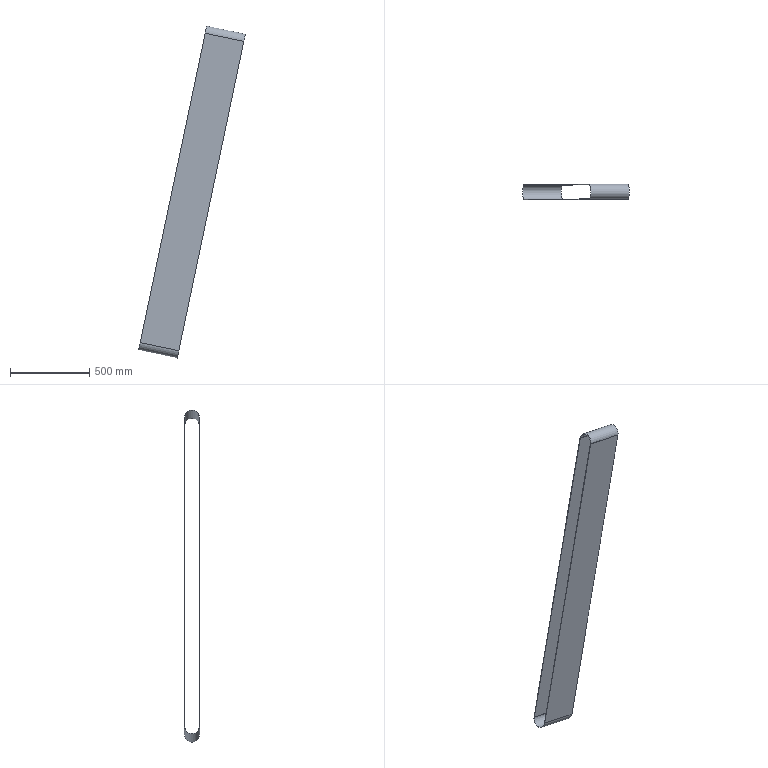Part | STEP file | ESTEIRA_002 | 1 solid | 10 faces | box 675.479 x 95 x 2102 mm | volume 2146084 mm3 | plane 6 | cylinder 4 | commonest cylinder face diameters 91 x2 95 x2
STEP:
#1=CARTESIAN_POINT('',(0.,0.,0.));
#2=DIRECTION('',(0.,0.,1.));
#3=DIRECTION('',(1.,0.,0.));
#4=AXIS2_PLACEMENT_3D('',#1,#2,#3);
#5=CARTESIAN_POINT('',(-4261.561,-580.65,1712.598));
#6=VERTEX_POINT('',#5);
#7=CARTESIAN_POINT('',(-4506.218,-580.65,1764.008));
#8=VERTEX_POINT('',#7);
#9=CARTESIAN_POINT('',(-4261.561,-580.65,1712.598));
#10=DIRECTION('',(-0.9786,0.,0.2056));
#11=VECTOR('',#10,1.);
#12=LINE('',#9,#11);
#13=CARTESIAN_POINT('',(-4383.89,-580.65,1738.303));
#14=DIRECTION('',(0.,1.,0.));
#15=DIRECTION('',(0.,0.,1.));
#16=AXIS2_PLACEMENT_3D('',#13,#14,#15);
#17=PLANE('',#16);
#18=CARTESIAN_POINT('',(-25.705,122.328));
#19=DIRECTION('',(0.2056,-0.9786));
#20=VECTOR('',#19,1.);
#21=LINE('',#18,#20);
#22=(GEOMETRIC_REPRESENTATION_CONTEXT(2)PARAMETRIC_REPRESENTATION_CONTEXT()REPRESENTATION_CONTEXT('',''));
#23=DEFINITIONAL_REPRESENTATION('',(#21),#22);
#24=PCURVE('',#17,#23);
#25=CARTESIAN_POINT('',(-4383.89,-628.15,1738.303));
#26=DIRECTION('',(0.9786,0.,-0.2056));
#27=DIRECTION('',(0.,1.,0.));
#28=AXIS2_PLACEMENT_3D('',#25,#26,#27);
#29=CYLINDRICAL_SURFACE('',#28,47.5);
#30=CARTESIAN_POINT('',(0.,125.));
#31=DIRECTION('',(0.,-1.));
#32=VECTOR('',#31,1.);
#33=LINE('',#30,#32);
#34=(GEOMETRIC_REPRESENTATION_CONTEXT(2)PARAMETRIC_REPRESENTATION_CONTEXT()REPRESENTATION_CONTEXT('',''));
#35=DEFINITIONAL_REPRESENTATION('',(#33),#34);
#36=PCURVE('',#29,#35);
#37=SURFACE_CURVE('',#12,(#24,#36),.PCURVE_S1.);
#38=EDGE_CURVE('',#6,#8,#37,.T.);
#39=ORIENTED_EDGE('',*,*,#38,.F.);
#40=CARTESIAN_POINT('',(-4672.848,-580.65,-244.657));
#41=VERTEX_POINT('',#40);
#42=CARTESIAN_POINT('',(-4261.561,-580.65,1712.598));
#43=DIRECTION('',(-0.2056,0.,-0.9786));
#44=VECTOR('',#43,1.);
#45=LINE('',#42,#44);
#46=CARTESIAN_POINT('',(-25.705,122.328));
#47=DIRECTION('',(-0.9786,-0.2056));
#48=VECTOR('',#47,1.);
#49=LINE('',#46,#48);
#50=(GEOMETRIC_REPRESENTATION_CONTEXT(2)PARAMETRIC_REPRESENTATION_CONTEXT()REPRESENTATION_CONTEXT('',''));
#51=DEFINITIONAL_REPRESENTATION('',(#49),#50);
#52=PCURVE('',#17,#51);
#53=CARTESIAN_POINT('',(-4426.,0.,930.055));
#54=DIRECTION('',(0.9786,0.,-0.2056));
#55=DIRECTION('',(-0.2056,0.,-0.9786));
#56=AXIS2_PLACEMENT_3D('',#53,#54,#55);
#57=PLANE('',#56);
#58=CARTESIAN_POINT('',(-799.633,-580.65));
#59=DIRECTION('',(1.,0.));
#60=VECTOR('',#59,1.);
#61=LINE('',#58,#60);
#62=(GEOMETRIC_REPRESENTATION_CONTEXT(2)PARAMETRIC_REPRESENTATION_CONTEXT()REPRESENTATION_CONTEXT('',''));
#63=DEFINITIONAL_REPRESENTATION('',(#61),#62);
#64=PCURVE('',#57,#63);
#65=SURFACE_CURVE('',#45,(#52,#64),.PCURVE_S1.);
#66=EDGE_CURVE('',#6,#41,#65,.T.);
#67=ORIENTED_EDGE('',*,*,#66,.T.);
#68=CARTESIAN_POINT('',(-4917.505,-580.65,-193.246));
#69=VERTEX_POINT('',#68);
#70=CARTESIAN_POINT('',(-4672.848,-580.65,-244.657));
#71=DIRECTION('',(-0.9786,0.,0.2056));
#72=VECTOR('',#71,1.);
#73=LINE('',#70,#72);
#74=CARTESIAN_POINT('',(-1982.959,-288.958));
#75=DIRECTION('',(0.2056,-0.9786));
#76=VECTOR('',#75,1.);
#77=LINE('',#74,#76);
#78=(GEOMETRIC_REPRESENTATION_CONTEXT(2)PARAMETRIC_REPRESENTATION_CONTEXT()REPRESENTATION_CONTEXT('',''));
#79=DEFINITIONAL_REPRESENTATION('',(#77),#78);
#80=PCURVE('',#17,#79);
#81=CARTESIAN_POINT('',(-4795.176,-628.15,-218.951));
#82=DIRECTION('',(0.9786,0.,-0.2056));
#83=DIRECTION('',(0.,-1.,0.));
#84=AXIS2_PLACEMENT_3D('',#81,#82,#83);
#85=CYLINDRICAL_SURFACE('',#84,47.5);
#86=CARTESIAN_POINT('',(3.142,125.));
#87=DIRECTION('',(0.,-1.));
#88=VECTOR('',#87,1.);
#89=LINE('',#86,#88);
#90=(GEOMETRIC_REPRESENTATION_CONTEXT(2)PARAMETRIC_REPRESENTATION_CONTEXT()REPRESENTATION_CONTEXT('',''));
#91=DEFINITIONAL_REPRESENTATION('',(#89),#90);
#92=PCURVE('',#85,#91);
#93=SURFACE_CURVE('',#73,(#80,#92),.PCURVE_S1.);
#94=EDGE_CURVE('',#41,#69,#93,.T.);
#95=ORIENTED_EDGE('',*,*,#94,.T.);
#96=CARTESIAN_POINT('',(-4506.218,-580.65,1764.008));
#97=DIRECTION('',(-0.2056,0.,-0.9786));
#98=VECTOR('',#97,1.);
#99=LINE('',#96,#98);
#100=CARTESIAN_POINT('',(25.705,-122.328));
#101=DIRECTION('',(-0.9786,-0.2056));
#102=VECTOR('',#101,1.);
#103=LINE('',#100,#102);
#104=(GEOMETRIC_REPRESENTATION_CONTEXT(2)PARAMETRIC_REPRESENTATION_CONTEXT()REPRESENTATION_CONTEXT('',''));
#105=DEFINITIONAL_REPRESENTATION('',(#103),#104);
#106=PCURVE('',#17,#105);
#107=CARTESIAN_POINT('',(-4670.657,0.,981.466));
#108=DIRECTION('',(0.9786,0.,-0.2056));
#109=DIRECTION('',(-0.2056,0.,-0.9786));
#110=AXIS2_PLACEMENT_3D('',#107,#108,#109);
#111=PLANE('',#110);
#112=CARTESIAN_POINT('',(-799.633,-580.65));
#113=DIRECTION('',(1.,0.));
#114=VECTOR('',#113,1.);
#115=LINE('',#112,#114);
#116=(GEOMETRIC_REPRESENTATION_CONTEXT(2)PARAMETRIC_REPRESENTATION_CONTEXT()REPRESENTATION_CONTEXT('',''));
#117=DEFINITIONAL_REPRESENTATION('',(#115),#116);
#118=PCURVE('',#111,#117);
#119=SURFACE_CURVE('',#99,(#106,#118),.PCURVE_S1.);
#120=EDGE_CURVE('',#8,#69,#119,.T.);
#121=ORIENTED_EDGE('',*,*,#120,.F.);
#122=EDGE_LOOP('',(#39,#67,#95,#121));
#123=FACE_BOUND('',#122,.T.);
#124=ADVANCED_FACE('',(#123),#17,.T.);
#125=CARTESIAN_POINT('',(-4506.218,-675.65,1764.008));
#126=VERTEX_POINT('',#125);
#127=CARTESIAN_POINT('',(-4506.218,-628.15,1764.008));
#128=DIRECTION('',(0.9786,0.,-0.2056));
#129=DIRECTION('',(0.2056,0.,0.9786));
#130=AXIS2_PLACEMENT_3D('',#127,#128,#129);
#131=CIRCLE('',#130,47.5);
#132=CARTESIAN_POINT('',(-4.712,-125.));
#133=DIRECTION('',(1.,0.));
#134=VECTOR('',#133,1.);
#135=LINE('',#132,#134);
#136=(GEOMETRIC_REPRESENTATION_CONTEXT(2)PARAMETRIC_REPRESENTATION_CONTEXT()REPRESENTATION_CONTEXT('',''));
#137=DEFINITIONAL_REPRESENTATION('',(#135),#136);
#138=PCURVE('',#29,#137);
#139=CARTESIAN_POINT('',(-799.633,-628.15));
#140=DIRECTION('',(-1.,0.));
#141=AXIS2_PLACEMENT_2D('',#139,#140);
#142=CIRCLE('',#141,47.5);
#143=(GEOMETRIC_REPRESENTATION_CONTEXT(2)PARAMETRIC_REPRESENTATION_CONTEXT()REPRESENTATION_CONTEXT('',''));
#144=DEFINITIONAL_REPRESENTATION('',(#142),#143);
#145=PCURVE('',#111,#144);
#146=SURFACE_CURVE('',#131,(#138,#145),.PCURVE_S1.);
#147=EDGE_CURVE('',#8,#126,#146,.T.);
#148=ORIENTED_EDGE('',*,*,#147,.T.);
#149=CARTESIAN_POINT('',(-4261.561,-675.65,1712.598));
#150=VERTEX_POINT('',#149);
#151=CARTESIAN_POINT('',(-4506.218,-675.65,1764.008));
#152=DIRECTION('',(0.9786,0.,-0.2056));
#153=VECTOR('',#152,1.);
#154=LINE('',#151,#153);
#155=CARTESIAN_POINT('',(3.142,-125.));
#156=DIRECTION('',(0.,1.));
#157=VECTOR('',#156,1.);
#158=LINE('',#155,#157);
#159=(GEOMETRIC_REPRESENTATION_CONTEXT(2)PARAMETRIC_REPRESENTATION_CONTEXT()REPRESENTATION_CONTEXT('',''));
#160=DEFINITIONAL_REPRESENTATION('',(#158),#159);
#161=PCURVE('',#29,#160);
#162=CARTESIAN_POINT('',(-4795.176,-675.65,-218.951));
#163=DIRECTION('',(0.,-1.,0.));
#164=DIRECTION('',(0.,0.,-1.));
#165=AXIS2_PLACEMENT_3D('',#162,#163,#164);
#166=PLANE('',#165);
#167=CARTESIAN_POINT('',(-1982.959,288.958));
#168=DIRECTION('',(0.2056,0.9786));
#169=VECTOR('',#168,1.);
#170=LINE('',#167,#169);
#171=(GEOMETRIC_REPRESENTATION_CONTEXT(2)PARAMETRIC_REPRESENTATION_CONTEXT()REPRESENTATION_CONTEXT('',''));
#172=DEFINITIONAL_REPRESENTATION('',(#170),#171);
#173=PCURVE('',#166,#172);
#174=SURFACE_CURVE('',#154,(#161,#173),.PCURVE_S1.);
#175=EDGE_CURVE('',#126,#150,#174,.T.);
#176=ORIENTED_EDGE('',*,*,#175,.T.);
#177=CARTESIAN_POINT('',(-4261.561,-628.15,1712.598));
#178=DIRECTION('',(0.9786,0.,-0.2056));
#179=DIRECTION('',(0.2056,0.,0.9786));
#180=AXIS2_PLACEMENT_3D('',#177,#178,#179);
#181=CIRCLE('',#180,47.5);
#182=CARTESIAN_POINT('',(-4.712,125.));
#183=DIRECTION('',(1.,0.));
#184=VECTOR('',#183,1.);
#185=LINE('',#182,#184);
#186=(GEOMETRIC_REPRESENTATION_CONTEXT(2)PARAMETRIC_REPRESENTATION_CONTEXT()REPRESENTATION_CONTEXT('',''));
#187=DEFINITIONAL_REPRESENTATION('',(#185),#186);
#188=PCURVE('',#29,#187);
#189=CARTESIAN_POINT('',(-799.633,-628.15));
#190=DIRECTION('',(-1.,0.));
#191=AXIS2_PLACEMENT_2D('',#189,#190);
#192=CIRCLE('',#191,47.5);
#193=(GEOMETRIC_REPRESENTATION_CONTEXT(2)PARAMETRIC_REPRESENTATION_CONTEXT()REPRESENTATION_CONTEXT('',''));
#194=DEFINITIONAL_REPRESENTATION('',(#192),#193);
#195=PCURVE('',#57,#194);
#196=SURFACE_CURVE('',#181,(#188,#195),.PCURVE_S1.);
#197=EDGE_CURVE('',#6,#150,#196,.T.);
#198=ORIENTED_EDGE('',*,*,#197,.F.);
#199=ORIENTED_EDGE('',*,*,#38,.T.);
#200=EDGE_LOOP('',(#148,#176,#198,#199));
#201=FACE_BOUND('',#200,.T.);
#202=ADVANCED_FACE('',(#201),#29,.T.);
#203=CARTESIAN_POINT('',(-4672.848,-675.65,-244.657));
#204=VERTEX_POINT('',#203);
#205=CARTESIAN_POINT('',(-4917.505,-675.65,-193.246));
#206=VERTEX_POINT('',#205);
#207=CARTESIAN_POINT('',(-4672.848,-675.65,-244.657));
#208=DIRECTION('',(-0.9786,0.,0.2056));
#209=VECTOR('',#208,1.);
#210=LINE('',#207,#209);
#211=CARTESIAN_POINT('',(25.705,122.328));
#212=DIRECTION('',(-0.2056,-0.9786));
#213=VECTOR('',#212,1.);
#214=LINE('',#211,#213);
#215=(GEOMETRIC_REPRESENTATION_CONTEXT(2)PARAMETRIC_REPRESENTATION_CONTEXT()REPRESENTATION_CONTEXT('',''));
#216=DEFINITIONAL_REPRESENTATION('',(#214),#215);
#217=PCURVE('',#166,#216);
#218=CARTESIAN_POINT('',(0.,125.));
#219=DIRECTION('',(0.,-1.));
#220=VECTOR('',#219,1.);
#221=LINE('',#218,#220);
#222=(GEOMETRIC_REPRESENTATION_CONTEXT(2)PARAMETRIC_REPRESENTATION_CONTEXT()REPRESENTATION_CONTEXT('',''));
#223=DEFINITIONAL_REPRESENTATION('',(#221),#222);
#224=PCURVE('',#85,#223);
#225=SURFACE_CURVE('',#210,(#217,#224),.PCURVE_S1.);
#226=EDGE_CURVE('',#204,#206,#225,.T.);
#227=ORIENTED_EDGE('',*,*,#226,.F.);
#228=CARTESIAN_POINT('',(-4672.848,-675.65,-244.657));
#229=DIRECTION('',(0.2056,0.,0.9786));
#230=VECTOR('',#229,1.);
#231=LINE('',#228,#230);
#232=CARTESIAN_POINT('',(25.705,122.328));
#233=DIRECTION('',(-0.9786,0.2056));
#234=VECTOR('',#233,1.);
#235=LINE('',#232,#234);
#236=(GEOMETRIC_REPRESENTATION_CONTEXT(2)PARAMETRIC_REPRESENTATION_CONTEXT()REPRESENTATION_CONTEXT('',''));
#237=DEFINITIONAL_REPRESENTATION('',(#235),#236);
#238=PCURVE('',#166,#237);
#239=CARTESIAN_POINT('',(1200.367,-675.65));
#240=DIRECTION('',(-1.,0.));
#241=VECTOR('',#240,1.);
#242=LINE('',#239,#241);
#243=(GEOMETRIC_REPRESENTATION_CONTEXT(2)PARAMETRIC_REPRESENTATION_CONTEXT()REPRESENTATION_CONTEXT('',''));
#244=DEFINITIONAL_REPRESENTATION('',(#242),#243);
#245=PCURVE('',#57,#244);
#246=SURFACE_CURVE('',#231,(#238,#245),.PCURVE_S1.);
#247=EDGE_CURVE('',#204,#150,#246,.T.);
#248=ORIENTED_EDGE('',*,*,#247,.T.);
#249=ORIENTED_EDGE('',*,*,#175,.F.);
#250=CARTESIAN_POINT('',(-4917.505,-675.65,-193.246));
#251=DIRECTION('',(0.2056,0.,0.9786));
#252=VECTOR('',#251,1.);
#253=LINE('',#250,#252);
#254=CARTESIAN_POINT('',(-25.705,-122.328));
#255=DIRECTION('',(-0.9786,0.2056));
#256=VECTOR('',#255,1.);
#257=LINE('',#254,#256);
#258=(GEOMETRIC_REPRESENTATION_CONTEXT(2)PARAMETRIC_REPRESENTATION_CONTEXT()REPRESENTATION_CONTEXT('',''));
#259=DEFINITIONAL_REPRESENTATION('',(#257),#258);
#260=PCURVE('',#166,#259);
#261=CARTESIAN_POINT('',(1200.367,-675.65));
#262=DIRECTION('',(-1.,0.));
#263=VECTOR('',#262,1.);
#264=LINE('',#261,#263);
#265=(GEOMETRIC_REPRESENTATION_CONTEXT(2)PARAMETRIC_REPRESENTATION_CONTEXT()REPRESENTATION_CONTEXT('',''));
#266=DEFINITIONAL_REPRESENTATION('',(#264),#265);
#267=PCURVE('',#111,#266);
#268=SURFACE_CURVE('',#253,(#260,#267),.PCURVE_S1.);
#269=EDGE_CURVE('',#206,#126,#268,.T.);
#270=ORIENTED_EDGE('',*,*,#269,.F.);
#271=EDGE_LOOP('',(#227,#248,#249,#270));
#272=FACE_BOUND('',#271,.T.);
#273=ADVANCED_FACE('',(#272),#166,.T.);
#274=CARTESIAN_POINT('',(-4917.505,-628.15,-193.246));
#275=DIRECTION('',(0.9786,0.,-0.2056));
#276=DIRECTION('',(0.2056,0.,0.9786));
#277=AXIS2_PLACEMENT_3D('',#274,#275,#276);
#278=CIRCLE('',#277,47.5);
#279=CARTESIAN_POINT('',(-1.571,-125.));
#280=DIRECTION('',(1.,0.));
#281=VECTOR('',#280,1.);
#282=LINE('',#279,#281);
#283=(GEOMETRIC_REPRESENTATION_CONTEXT(2)PARAMETRIC_REPRESENTATION_CONTEXT()REPRESENTATION_CONTEXT('',''));
#284=DEFINITIONAL_REPRESENTATION('',(#282),#283);
#285=PCURVE('',#85,#284);
#286=CARTESIAN_POINT('',(1200.367,-628.15));
#287=DIRECTION('',(-1.,0.));
#288=AXIS2_PLACEMENT_2D('',#286,#287);
#289=CIRCLE('',#288,47.5);
#290=(GEOMETRIC_REPRESENTATION_CONTEXT(2)PARAMETRIC_REPRESENTATION_CONTEXT()REPRESENTATION_CONTEXT('',''));
#291=DEFINITIONAL_REPRESENTATION('',(#289),#290);
#292=PCURVE('',#111,#291);
#293=SURFACE_CURVE('',#278,(#285,#292),.PCURVE_S1.);
#294=EDGE_CURVE('',#206,#69,#293,.T.);
#295=ORIENTED_EDGE('',*,*,#294,.T.);
#296=ORIENTED_EDGE('',*,*,#94,.F.);
#297=CARTESIAN_POINT('',(-4672.848,-628.15,-244.657));
#298=DIRECTION('',(0.9786,0.,-0.2056));
#299=DIRECTION('',(0.2056,0.,0.9786));
#300=AXIS2_PLACEMENT_3D('',#297,#298,#299);
#301=CIRCLE('',#300,47.5);
#302=CARTESIAN_POINT('',(-1.571,125.));
#303=DIRECTION('',(1.,0.));
#304=VECTOR('',#303,1.);
#305=LINE('',#302,#304);
#306=(GEOMETRIC_REPRESENTATION_CONTEXT(2)PARAMETRIC_REPRESENTATION_CONTEXT()REPRESENTATION_CONTEXT('',''));
#307=DEFINITIONAL_REPRESENTATION('',(#305),#306);
#308=PCURVE('',#85,#307);
#309=CARTESIAN_POINT('',(1200.367,-628.15));
#310=DIRECTION('',(-1.,0.));
#311=AXIS2_PLACEMENT_2D('',#309,#310);
#312=CIRCLE('',#311,47.5);
#313=(GEOMETRIC_REPRESENTATION_CONTEXT(2)PARAMETRIC_REPRESENTATION_CONTEXT()REPRESENTATION_CONTEXT('',''));
#314=DEFINITIONAL_REPRESENTATION('',(#312),#313);
#315=PCURVE('',#57,#314);
#316=SURFACE_CURVE('',#301,(#308,#315),.PCURVE_S1.);
#317=EDGE_CURVE('',#204,#41,#316,.T.);
#318=ORIENTED_EDGE('',*,*,#317,.F.);
#319=ORIENTED_EDGE('',*,*,#226,.T.);
#320=EDGE_LOOP('',(#295,#296,#318,#319));
#321=FACE_BOUND('',#320,.T.);
#322=ADVANCED_FACE('',(#321),#85,.T.);
#323=CARTESIAN_POINT('',(-4506.218,-582.65,1764.008));
#324=VERTEX_POINT('',#323);
#325=CARTESIAN_POINT('',(-4917.505,-582.65,-193.246));
#326=VERTEX_POINT('',#325);
#327=CARTESIAN_POINT('',(-4506.218,-582.65,1764.008));
#328=DIRECTION('',(-0.2056,0.,-0.9786));
#329=VECTOR('',#328,1.);
#330=LINE('',#327,#329);
#331=CARTESIAN_POINT('',(-4383.89,-582.65,1738.303));
#332=DIRECTION('',(0.,1.,0.));
#333=DIRECTION('',(0.,0.,1.));
#334=AXIS2_PLACEMENT_3D('',#331,#332,#333);
#335=PLANE('',#334);
#336=CARTESIAN_POINT('',(25.705,-122.328));
#337=DIRECTION('',(-0.9786,-0.2056));
#338=VECTOR('',#337,1.);
#339=LINE('',#336,#338);
#340=(GEOMETRIC_REPRESENTATION_CONTEXT(2)PARAMETRIC_REPRESENTATION_CONTEXT()REPRESENTATION_CONTEXT('',''));
#341=DEFINITIONAL_REPRESENTATION('',(#339),#340);
#342=PCURVE('',#335,#341);
#343=CARTESIAN_POINT('',(-799.633,-582.65));
#344=DIRECTION('',(1.,0.));
#345=VECTOR('',#344,1.);
#346=LINE('',#343,#345);
#347=(GEOMETRIC_REPRESENTATION_CONTEXT(2)PARAMETRIC_REPRESENTATION_CONTEXT()REPRESENTATION_CONTEXT('',''));
#348=DEFINITIONAL_REPRESENTATION('',(#346),#347);
#349=PCURVE('',#111,#348);
#350=SURFACE_CURVE('',#330,(#342,#349),.PCURVE_S1.);
#351=EDGE_CURVE('',#324,#326,#350,.T.);
#352=ORIENTED_EDGE('',*,*,#351,.T.);
#353=CARTESIAN_POINT('',(-4672.848,-582.65,-244.657));
#354=VERTEX_POINT('',#353);
#355=CARTESIAN_POINT('',(-4672.848,-582.65,-244.657));
#356=DIRECTION('',(-0.9786,0.,0.2056));
#357=VECTOR('',#356,1.);
#358=LINE('',#355,#357);
#359=CARTESIAN_POINT('',(-1982.959,-288.958));
#360=DIRECTION('',(0.2056,-0.9786));
#361=VECTOR('',#360,1.);
#362=LINE('',#359,#361);
#363=(GEOMETRIC_REPRESENTATION_CONTEXT(2)PARAMETRIC_REPRESENTATION_CONTEXT()REPRESENTATION_CONTEXT('',''));
#364=DEFINITIONAL_REPRESENTATION('',(#362),#363);
#365=PCURVE('',#335,#364);
#366=CARTESIAN_POINT('',(-4795.176,-628.15,-218.951));
#367=DIRECTION('',(0.9786,0.,-0.2056));
#368=DIRECTION('',(0.,-1.,0.));
#369=AXIS2_PLACEMENT_3D('',#366,#367,#368);
#370=CYLINDRICAL_SURFACE('',#369,45.5);
#371=CARTESIAN_POINT('',(3.142,125.));
#372=DIRECTION('',(0.,-1.));
#373=VECTOR('',#372,1.);
#374=LINE('',#371,#373);
#375=(GEOMETRIC_REPRESENTATION_CONTEXT(2)PARAMETRIC_REPRESENTATION_CONTEXT()REPRESENTATION_CONTEXT('',''));
#376=DEFINITIONAL_REPRESENTATION('',(#374),#375);
#377=PCURVE('',#370,#376);
#378=SURFACE_CURVE('',#358,(#365,#377),.PCURVE_S1.);
#379=EDGE_CURVE('',#354,#326,#378,.T.);
#380=ORIENTED_EDGE('',*,*,#379,.F.);
#381=CARTESIAN_POINT('',(-4261.561,-582.65,1712.598));
#382=VERTEX_POINT('',#381);
#383=CARTESIAN_POINT('',(-4261.561,-582.65,1712.598));
#384=DIRECTION('',(-0.2056,0.,-0.9786));
#385=VECTOR('',#384,1.);
#386=LINE('',#383,#385);
#387=CARTESIAN_POINT('',(-25.705,122.328));
#388=DIRECTION('',(-0.9786,-0.2056));
#389=VECTOR('',#388,1.);
#390=LINE('',#387,#389);
#391=(GEOMETRIC_REPRESENTATION_CONTEXT(2)PARAMETRIC_REPRESENTATION_CONTEXT()REPRESENTATION_CONTEXT('',''));
#392=DEFINITIONAL_REPRESENTATION('',(#390),#391);
#393=PCURVE('',#335,#392);
#394=CARTESIAN_POINT('',(-799.633,-582.65));
#395=DIRECTION('',(1.,0.));
#396=VECTOR('',#395,1.);
#397=LINE('',#394,#396);
#398=(GEOMETRIC_REPRESENTATION_CONTEXT(2)PARAMETRIC_REPRESENTATION_CONTEXT()REPRESENTATION_CONTEXT('',''));
#399=DEFINITIONAL_REPRESENTATION('',(#397),#398);
#400=PCURVE('',#57,#399);
#401=SURFACE_CURVE('',#386,(#393,#400),.PCURVE_S1.);
#402=EDGE_CURVE('',#382,#354,#401,.T.);
#403=ORIENTED_EDGE('',*,*,#402,.F.);
#404=CARTESIAN_POINT('',(-4261.561,-582.65,1712.598));
#405=DIRECTION('',(-0.9786,0.,0.2056));
#406=VECTOR('',#405,1.);
#407=LINE('',#404,#406);
#408=CARTESIAN_POINT('',(-25.705,122.328));
#409=DIRECTION('',(0.2056,-0.9786));
#410=VECTOR('',#409,1.);
#411=LINE('',#408,#410);
#412=(GEOMETRIC_REPRESENTATION_CONTEXT(2)PARAMETRIC_REPRESENTATION_CONTEXT()REPRESENTATION_CONTEXT('',''));
#413=DEFINITIONAL_REPRESENTATION('',(#411),#412);
#414=PCURVE('',#335,#413);
#415=CARTESIAN_POINT('',(-4383.89,-628.15,1738.303));
#416=DIRECTION('',(0.9786,0.,-0.2056));
#417=DIRECTION('',(0.,1.,0.));
#418=AXIS2_PLACEMENT_3D('',#415,#416,#417);
#419=CYLINDRICAL_SURFACE('',#418,45.5);
#420=CARTESIAN_POINT('',(0.,125.));
#421=DIRECTION('',(0.,-1.));
#422=VECTOR('',#421,1.);
#423=LINE('',#420,#422);
#424=(GEOMETRIC_REPRESENTATION_CONTEXT(2)PARAMETRIC_REPRESENTATION_CONTEXT()REPRESENTATION_CONTEXT('',''));
#425=DEFINITIONAL_REPRESENTATION('',(#423),#424);
#426=PCURVE('',#419,#425);
#427=SURFACE_CURVE('',#407,(#414,#426),.PCURVE_S1.);
#428=EDGE_CURVE('',#382,#324,#427,.T.);
#429=ORIENTED_EDGE('',*,*,#428,.T.);
#430=EDGE_LOOP('',(#352,#380,#403,#429));
#431=FACE_BOUND('',#430,.T.);
#432=ADVANCED_FACE('',(#431),#335,.F.);
#433=CARTESIAN_POINT('',(-4917.505,-673.65,-193.246));
#434=VERTEX_POINT('',#433);
#435=CARTESIAN_POINT('',(-4917.505,-628.15,-193.246));
#436=DIRECTION('',(0.9786,0.,-0.2056));
#437=DIRECTION('',(0.2056,0.,0.9786));
#438=AXIS2_PLACEMENT_3D('',#435,#436,#437);
#439=CIRCLE('',#438,45.5);
#440=CARTESIAN_POINT('',(-1.571,-125.));
#441=DIRECTION('',(1.,0.));
#442=VECTOR('',#441,1.);
#443=LINE('',#440,#442);
#444=(GEOMETRIC_REPRESENTATION_CONTEXT(2)PARAMETRIC_REPRESENTATION_CONTEXT()REPRESENTATION_CONTEXT('',''));
#445=DEFINITIONAL_REPRESENTATION('',(#443),#444);
#446=PCURVE('',#370,#445);
#447=CARTESIAN_POINT('',(1200.367,-628.15));
#448=DIRECTION('',(-1.,0.));
#449=AXIS2_PLACEMENT_2D('',#447,#448);
#450=CIRCLE('',#449,45.5);
#451=(GEOMETRIC_REPRESENTATION_CONTEXT(2)PARAMETRIC_REPRESENTATION_CONTEXT()REPRESENTATION_CONTEXT('',''));
#452=DEFINITIONAL_REPRESENTATION('',(#450),#451);
#453=PCURVE('',#111,#452);
#454=SURFACE_CURVE('',#439,(#446,#453),.PCURVE_S1.);
#455=EDGE_CURVE('',#434,#326,#454,.T.);
#456=ORIENTED_EDGE('',*,*,#455,.T.);
#457=ORIENTED_EDGE('',*,*,#379,.F.);
#458=CARTESIAN_POINT('',(-4672.848,-673.65,-244.657));
#459=VERTEX_POINT('',#458);
#460=CARTESIAN_POINT('',(-4672.848,-628.15,-244.657));
#461=DIRECTION('',(0.9786,0.,-0.2056));
#462=DIRECTION('',(0.2056,0.,0.9786));
#463=AXIS2_PLACEMENT_3D('',#460,#461,#462);
#464=CIRCLE('',#463,45.5);
#465=CARTESIAN_POINT('',(-1.571,125.));
#466=DIRECTION('',(1.,0.));
#467=VECTOR('',#466,1.);
#468=LINE('',#465,#467);
#469=(GEOMETRIC_REPRESENTATION_CONTEXT(2)PARAMETRIC_REPRESENTATION_CONTEXT()REPRESENTATION_CONTEXT('',''));
#470=DEFINITIONAL_REPRESENTATION('',(#468),#469);
#471=PCURVE('',#370,#470);
#472=CARTESIAN_POINT('',(1200.367,-628.15));
#473=DIRECTION('',(-1.,0.));
#474=AXIS2_PLACEMENT_2D('',#472,#473);
#475=CIRCLE('',#474,45.5);
#476=(GEOMETRIC_REPRESENTATION_CONTEXT(2)PARAMETRIC_REPRESENTATION_CONTEXT()REPRESENTATION_CONTEXT('',''));
#477=DEFINITIONAL_REPRESENTATION('',(#475),#476);
#478=PCURVE('',#57,#477);
#479=SURFACE_CURVE('',#464,(#471,#478),.PCURVE_S1.);
#480=EDGE_CURVE('',#459,#354,#479,.T.);
#481=ORIENTED_EDGE('',*,*,#480,.F.);
#482=CARTESIAN_POINT('',(-4917.505,-673.65,-193.246));
#483=DIRECTION('',(0.9786,0.,-0.2056));
#484=VECTOR('',#483,1.);
#485=LINE('',#482,#484);
#486=CARTESIAN_POINT('',(0.,-125.));
#487=DIRECTION('',(0.,1.));
#488=VECTOR('',#487,1.);
#489=LINE('',#486,#488);
#490=(GEOMETRIC_REPRESENTATION_CONTEXT(2)PARAMETRIC_REPRESENTATION_CONTEXT()REPRESENTATION_CONTEXT('',''));
#491=DEFINITIONAL_REPRESENTATION('',(#489),#490);
#492=PCURVE('',#370,#491);
#493=CARTESIAN_POINT('',(-4795.176,-673.65,-218.951));
#494=DIRECTION('',(0.,-1.,0.));
#495=DIRECTION('',(0.,0.,-1.));
#496=AXIS2_PLACEMENT_3D('',#493,#494,#495);
#497=PLANE('',#496);
#498=CARTESIAN_POINT('',(-25.705,-122.328));
#499=DIRECTION('',(0.2056,0.9786));
#500=VECTOR('',#499,1.);
#501=LINE('',#498,#500);
#502=(GEOMETRIC_REPRESENTATION_CONTEXT(2)PARAMETRIC_REPRESENTATION_CONTEXT()REPRESENTATION_CONTEXT('',''));
#503=DEFINITIONAL_REPRESENTATION('',(#501),#502);
#504=PCURVE('',#497,#503);
#505=SURFACE_CURVE('',#485,(#492,#504),.PCURVE_S1.);
#506=EDGE_CURVE('',#434,#459,#505,.T.);
#507=ORIENTED_EDGE('',*,*,#506,.F.);
#508=EDGE_LOOP('',(#456,#457,#481,#507));
#509=FACE_BOUND('',#508,.F.);
#510=ADVANCED_FACE('',(#509),#370,.F.);
#511=CARTESIAN_POINT('',(-4506.218,-673.65,1764.008));
#512=VERTEX_POINT('',#511);
#513=CARTESIAN_POINT('',(-4917.505,-673.65,-193.246));
#514=DIRECTION('',(0.2056,0.,0.9786));
#515=VECTOR('',#514,1.);
#516=LINE('',#513,#515);
#517=CARTESIAN_POINT('',(-25.705,-122.328));
#518=DIRECTION('',(-0.9786,0.2056));
#519=VECTOR('',#518,1.);
#520=LINE('',#517,#519);
#521=(GEOMETRIC_REPRESENTATION_CONTEXT(2)PARAMETRIC_REPRESENTATION_CONTEXT()REPRESENTATION_CONTEXT('',''));
#522=DEFINITIONAL_REPRESENTATION('',(#520),#521);
#523=PCURVE('',#497,#522);
#524=CARTESIAN_POINT('',(1200.367,-673.65));
#525=DIRECTION('',(-1.,0.));
#526=VECTOR('',#525,1.);
#527=LINE('',#524,#526);
#528=(GEOMETRIC_REPRESENTATION_CONTEXT(2)PARAMETRIC_REPRESENTATION_CONTEXT()REPRESENTATION_CONTEXT('',''));
#529=DEFINITIONAL_REPRESENTATION('',(#527),#528);
#530=PCURVE('',#111,#529);
#531=SURFACE_CURVE('',#516,(#523,#530),.PCURVE_S1.);
#532=EDGE_CURVE('',#434,#512,#531,.T.);
#533=ORIENTED_EDGE('',*,*,#532,.T.);
#534=CARTESIAN_POINT('',(-4261.561,-673.65,1712.598));
#535=VERTEX_POINT('',#534);
#536=CARTESIAN_POINT('',(-4261.561,-673.65,1712.598));
#537=DIRECTION('',(-0.9786,0.,0.2056));
#538=VECTOR('',#537,1.);
#539=LINE('',#536,#538);
#540=CARTESIAN_POINT('',(-1931.549,533.615));
#541=DIRECTION('',(-0.2056,-0.9786));
#542=VECTOR('',#541,1.);
#543=LINE('',#540,#542);
#544=(GEOMETRIC_REPRESENTATION_CONTEXT(2)PARAMETRIC_REPRESENTATION_CONTEXT()REPRESENTATION_CONTEXT('',''));
#545=DEFINITIONAL_REPRESENTATION('',(#543),#544);
#546=PCURVE('',#497,#545);
#547=CARTESIAN_POINT('',(3.142,125.));
#548=DIRECTION('',(0.,-1.));
#549=VECTOR('',#548,1.);
#550=LINE('',#547,#549);
#551=(GEOMETRIC_REPRESENTATION_CONTEXT(2)PARAMETRIC_REPRESENTATION_CONTEXT()REPRESENTATION_CONTEXT('',''));
#552=DEFINITIONAL_REPRESENTATION('',(#550),#551);
#553=PCURVE('',#419,#552);
#554=SURFACE_CURVE('',#539,(#546,#553),.PCURVE_S1.);
#555=EDGE_CURVE('',#535,#512,#554,.T.);
#556=ORIENTED_EDGE('',*,*,#555,.F.);
#557=CARTESIAN_POINT('',(-4672.848,-673.65,-244.657));
#558=DIRECTION('',(0.2056,0.,0.9786));
#559=VECTOR('',#558,1.);
#560=LINE('',#557,#559);
#561=CARTESIAN_POINT('',(25.705,122.328));
#562=DIRECTION('',(-0.9786,0.2056));
#563=VECTOR('',#562,1.);
#564=LINE('',#561,#563);
#565=(GEOMETRIC_REPRESENTATION_CONTEXT(2)PARAMETRIC_REPRESENTATION_CONTEXT()REPRESENTATION_CONTEXT('',''));
#566=DEFINITIONAL_REPRESENTATION('',(#564),#565);
#567=PCURVE('',#497,#566);
#568=CARTESIAN_POINT('',(1200.367,-673.65));
#569=DIRECTION('',(-1.,0.));
#570=VECTOR('',#569,1.);
#571=LINE('',#568,#570);
#572=(GEOMETRIC_REPRESENTATION_CONTEXT(2)PARAMETRIC_REPRESENTATION_CONTEXT()REPRESENTATION_CONTEXT('',''));
#573=DEFINITIONAL_REPRESENTATION('',(#571),#572);
#574=PCURVE('',#57,#573);
#575=SURFACE_CURVE('',#560,(#567,#574),.PCURVE_S1.);
#576=EDGE_CURVE('',#459,#535,#575,.T.);
#577=ORIENTED_EDGE('',*,*,#576,.F.);
#578=ORIENTED_EDGE('',*,*,#506,.F.);
#579=EDGE_LOOP('',(#533,#556,#577,#578));
#580=FACE_BOUND('',#579,.T.);
#581=ADVANCED_FACE('',(#580),#497,.F.);
#582=CARTESIAN_POINT('',(-4506.218,-628.15,1764.008));
#583=DIRECTION('',(0.9786,0.,-0.2056));
#584=DIRECTION('',(0.2056,0.,0.9786));
#585=AXIS2_PLACEMENT_3D('',#582,#583,#584);
#586=CIRCLE('',#585,45.5);
#587=CARTESIAN_POINT('',(-4.712,-125.));
#588=DIRECTION('',(1.,0.));
#589=VECTOR('',#588,1.);
#590=LINE('',#587,#589);
#591=(GEOMETRIC_REPRESENTATION_CONTEXT(2)PARAMETRIC_REPRESENTATION_CONTEXT()REPRESENTATION_CONTEXT('',''));
#592=DEFINITIONAL_REPRESENTATION('',(#590),#591);
#593=PCURVE('',#419,#592);
#594=CARTESIAN_POINT('',(-799.633,-628.15));
#595=DIRECTION('',(-1.,0.));
#596=AXIS2_PLACEMENT_2D('',#594,#595);
#597=CIRCLE('',#596,45.5);
#598=(GEOMETRIC_REPRESENTATION_CONTEXT(2)PARAMETRIC_REPRESENTATION_CONTEXT()REPRESENTATION_CONTEXT('',''));
#599=DEFINITIONAL_REPRESENTATION('',(#597),#598);
#600=PCURVE('',#111,#599);
#601=SURFACE_CURVE('',#586,(#593,#600),.PCURVE_S1.);
#602=EDGE_CURVE('',#324,#512,#601,.T.);
#603=ORIENTED_EDGE('',*,*,#602,.T.);
#604=ORIENTED_EDGE('',*,*,#555,.F.);
#605=CARTESIAN_POINT('',(-4261.561,-628.15,1712.598));
#606=DIRECTION('',(0.9786,0.,-0.2056));
#607=DIRECTION('',(0.2056,0.,0.9786));
#608=AXIS2_PLACEMENT_3D('',#605,#606,#607);
#609=CIRCLE('',#608,45.5);
#610=CARTESIAN_POINT('',(-4.712,125.));
#611=DIRECTION('',(1.,0.));
#612=VECTOR('',#611,1.);
#613=LINE('',#610,#612);
#614=(GEOMETRIC_REPRESENTATION_CONTEXT(2)PARAMETRIC_REPRESENTATION_CONTEXT()REPRESENTATION_CONTEXT('',''));
#615=DEFINITIONAL_REPRESENTATION('',(#613),#614);
#616=PCURVE('',#419,#615);
#617=CARTESIAN_POINT('',(-799.633,-628.15));
#618=DIRECTION('',(-1.,0.));
#619=AXIS2_PLACEMENT_2D('',#617,#618);
#620=CIRCLE('',#619,45.5);
#621=(GEOMETRIC_REPRESENTATION_CONTEXT(2)PARAMETRIC_REPRESENTATION_CONTEXT()REPRESENTATION_CONTEXT('',''));
#622=DEFINITIONAL_REPRESENTATION('',(#620),#621);
#623=PCURVE('',#57,#622);
#624=SURFACE_CURVE('',#609,(#616,#623),.PCURVE_S1.);
#625=EDGE_CURVE('',#382,#535,#624,.T.);
#626=ORIENTED_EDGE('',*,*,#625,.F.);
#627=ORIENTED_EDGE('',*,*,#428,.T.);
#628=EDGE_LOOP('',(#603,#604,#626,#627));
#629=FACE_BOUND('',#628,.F.);
#630=ADVANCED_FACE('',(#629),#419,.F.);
#631=ORIENTED_EDGE('',*,*,#66,.F.);
#632=ORIENTED_EDGE('',*,*,#197,.T.);
#633=ORIENTED_EDGE('',*,*,#247,.F.);
#634=ORIENTED_EDGE('',*,*,#317,.T.);
#635=EDGE_LOOP('',(#631,#632,#633,#634));
#636=FACE_BOUND('',#635,.T.);
#637=ORIENTED_EDGE('',*,*,#402,.T.);
#638=ORIENTED_EDGE('',*,*,#480,.F.);
#639=ORIENTED_EDGE('',*,*,#576,.T.);
#640=ORIENTED_EDGE('',*,*,#625,.F.);
#641=EDGE_LOOP('',(#637,#638,#639,#640));
#642=FACE_BOUND('',#641,.T.);
#643=ADVANCED_FACE('',(#636,#642),#57,.T.);
#644=ORIENTED_EDGE('',*,*,#294,.F.);
#645=ORIENTED_EDGE('',*,*,#269,.T.);
#646=ORIENTED_EDGE('',*,*,#147,.F.);
#647=ORIENTED_EDGE('',*,*,#120,.T.);
#648=EDGE_LOOP('',(#644,#645,#646,#647));
#649=FACE_BOUND('',#648,.T.);
#650=ORIENTED_EDGE('',*,*,#602,.T.);
#651=ORIENTED_EDGE('',*,*,#532,.F.);
#652=ORIENTED_EDGE('',*,*,#455,.T.);
#653=ORIENTED_EDGE('',*,*,#351,.F.);
#654=EDGE_LOOP('',(#650,#651,#652,#653));
#655=FACE_BOUND('',#654,.T.);
#656=ADVANCED_FACE('',(#649,#655),#111,.F.);
#657=CLOSED_SHELL('',(#124,#202,#273,#322,#432,#510,#581,#630,#643,#656));
#658=MANIFOLD_SOLID_BREP('',#657);
#659=(LENGTH_UNIT()NAMED_UNIT(*)SI_UNIT(.MILLI.,.METRE.));
#660=UNCERTAINTY_MEASURE_WITH_UNIT(LENGTH_MEASURE(0.0000001),#659,'','');
#661=(NAMED_UNIT(*)PLANE_ANGLE_UNIT()SI_UNIT($,.RADIAN.));
#662=(NAMED_UNIT(*)SI_UNIT($,.STERADIAN.)SOLID_ANGLE_UNIT());
#663=(GEOMETRIC_REPRESENTATION_CONTEXT(3)GLOBAL_UNCERTAINTY_ASSIGNED_CONTEXT((#660))GLOBAL_UNIT_ASSIGNED_CONTEXT((#659,#661,#662))REPRESENTATION_CONTEXT('',''));
#664=ADVANCED_BREP_SHAPE_REPRESENTATION('',(#4,#658),#663);